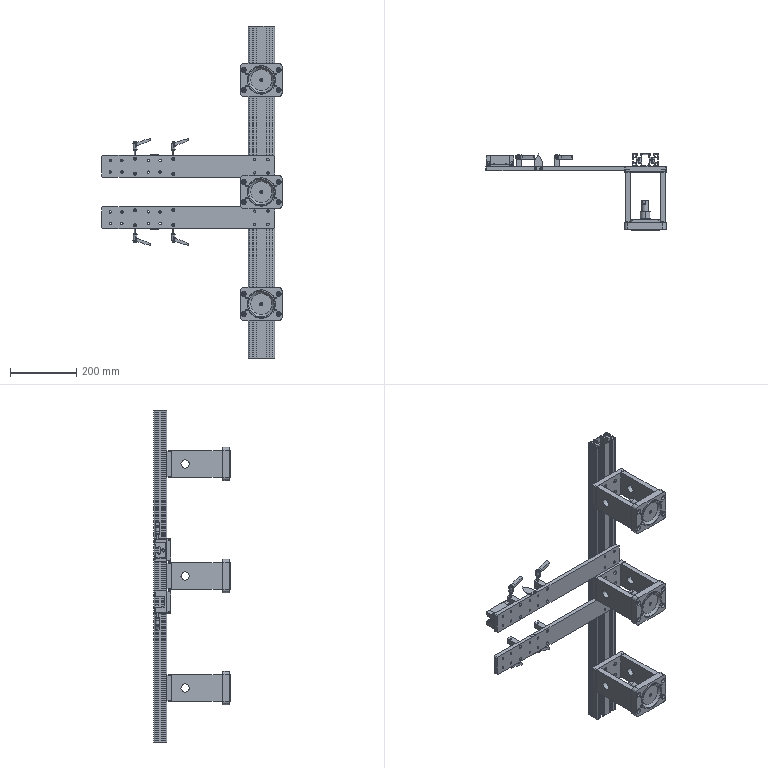Part | SolidWorks | features ReferencePattern 11, LocalLPattern 2, MirrorCompFeat 2 | 43 solids | 1482 faces | box 542.5 x 231.5 x 1000 mm | volume 4307591 mm3 | plane 663 | cylinder 628 | cone 183 | torus 8 | commonest cylinder face diameters 6.8 x64 5 x48 6.6 x48 7 x48 15 x48 9 x40